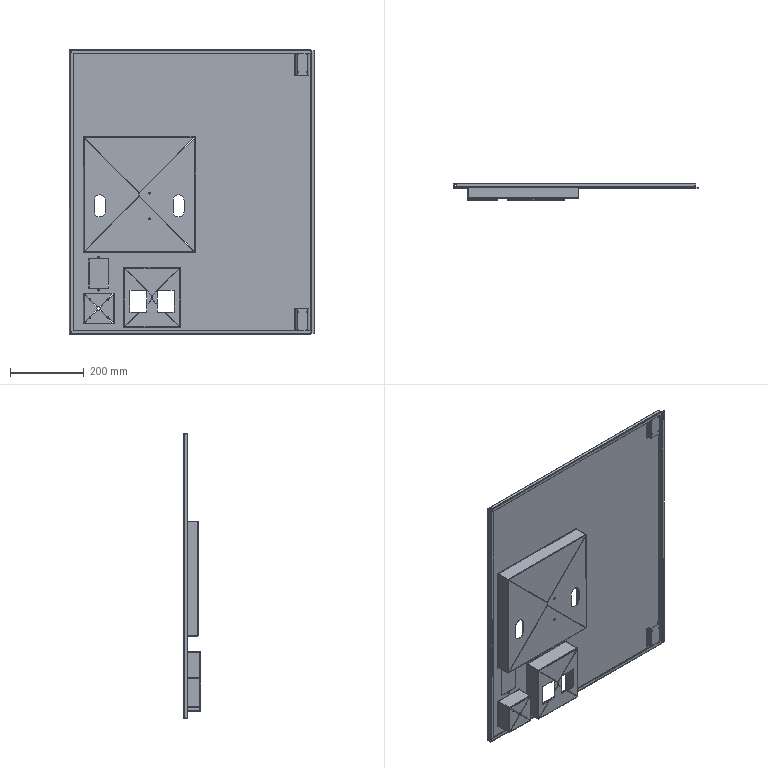Part | SolidWorks | features EdgeFlange 8, ICE 6, FlatPattern 5, HoleWzd 3, SMBaseFlange 2, SMWeldBead 2, SheetMetal 2, MirrorPattern 1, MirrorSolid 1 | 5 solids | 493 faces | box 667.5 x 46.5 x 774 mm | volume 968316 mm3 | plane 286 | cylinder 135 | spline 72 | commonest cylinder face diameters 1 x31 4 x31 2.5 x20 4.2 x12 6 x12 2 x10